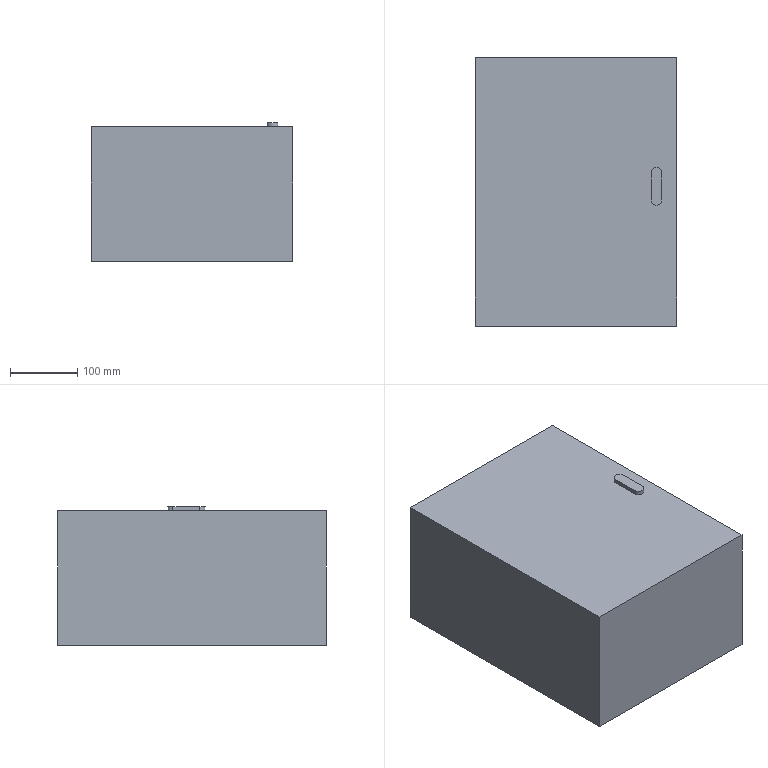Part | SolidWorks | features Extrusion 1, ICE 1 | 1 solid | 11 faces | box 300 x 400 x 206 mm | volume 24005084 mm3 | plane 9 | cylinder 2 | commonest cylinder face diameters 16.06 x2
STEP:
#1=CARTESIAN_POINT('',(-150.,200.,100.));
#2=VERTEX_POINT('',#1);
#3=CARTESIAN_POINT('',(-150.,-200.,100.));
#4=VERTEX_POINT('',#3);
#5=CARTESIAN_POINT('',(-150.,-200.,100.));
#6=DIRECTION('',(0.,-1.,0.));
#7=VECTOR('',#6,1000.);
#8=LINE('',#5,#7);
#9=EDGE_CURVE('',#2,#4,#8,.T.);
#10=ORIENTED_EDGE('',*,*,#9,.T.);
#11=CARTESIAN_POINT('',(150.,-200.,100.));
#12=VERTEX_POINT('',#11);
#13=CARTESIAN_POINT('',(150.,-200.,100.));
#14=DIRECTION('',(1.,0.,0.));
#15=VECTOR('',#14,1000.);
#16=LINE('',#13,#15);
#17=EDGE_CURVE('',#4,#12,#16,.T.);
#18=ORIENTED_EDGE('',*,*,#17,.T.);
#19=CARTESIAN_POINT('',(150.,200.,100.));
#20=VERTEX_POINT('',#19);
#21=CARTESIAN_POINT('',(150.,-200.,100.));
#22=DIRECTION('',(0.,1.,0.));
#23=VECTOR('',#22,1000.);
#24=LINE('',#21,#23);
#25=EDGE_CURVE('',#12,#20,#24,.T.);
#26=ORIENTED_EDGE('',*,*,#25,.T.);
#27=CARTESIAN_POINT('',(150.,200.,100.));
#28=DIRECTION('',(-1.,0.,0.));
#29=VECTOR('',#28,1000.);
#30=LINE('',#27,#29);
#31=EDGE_CURVE('',#20,#2,#30,.T.);
#32=ORIENTED_EDGE('',*,*,#31,.T.);
#33=EDGE_LOOP('',(#10,#18,#26,#32));
#34=FACE_OUTER_BOUND('',#33,.T.);
#35=CARTESIAN_POINT('',(111.97,28.454,100.));
#36=VERTEX_POINT('',#35);
#37=CARTESIAN_POINT('',(111.97,-11.696,100.));
#38=VERTEX_POINT('',#37);
#39=CARTESIAN_POINT('',(111.97,28.454,100.));
#40=DIRECTION('',(0.,-1.,0.));
#41=VECTOR('',#40,1000.);
#42=LINE('',#39,#41);
#43=EDGE_CURVE('',#36,#38,#42,.T.);
#44=ORIENTED_EDGE('',*,*,#43,.F.);
#45=CARTESIAN_POINT('',(128.03,28.454,100.));
#46=VERTEX_POINT('',#45);
#47=CARTESIAN_POINT('',(120.,28.454,100.));
#48=DIRECTION('',(0.,0.,1.));
#49=DIRECTION('',(1.,0.,0.));
#50=AXIS2_PLACEMENT_3D('',#47,#48,#49);
#51=CIRCLE('',#50,8.03);
#52=EDGE_CURVE('',#46,#36,#51,.T.);
#53=ORIENTED_EDGE('',*,*,#52,.F.);
#54=CARTESIAN_POINT('',(128.03,-11.696,100.));
#55=VERTEX_POINT('',#54);
#56=CARTESIAN_POINT('',(128.03,28.454,100.));
#57=DIRECTION('',(0.,1.,0.));
#58=VECTOR('',#57,1000.);
#59=LINE('',#56,#58);
#60=EDGE_CURVE('',#55,#46,#59,.T.);
#61=ORIENTED_EDGE('',*,*,#60,.F.);
#62=CARTESIAN_POINT('',(120.,-11.696,100.));
#63=DIRECTION('',(0.,0.,1.));
#64=DIRECTION('',(1.,0.,0.));
#65=AXIS2_PLACEMENT_3D('',#62,#63,#64);
#66=CIRCLE('',#65,8.03);
#67=EDGE_CURVE('',#38,#55,#66,.T.);
#68=ORIENTED_EDGE('',*,*,#67,.F.);
#69=EDGE_LOOP('',(#44,#53,#61,#68));
#70=FACE_BOUND('',#69,.T.);
#71=CARTESIAN_POINT('',(0.,0.,100.));
#72=DIRECTION('',(0.,0.,1.));
#73=DIRECTION('',(1.,0.,0.));
#74=AXIS2_PLACEMENT_3D('',#71,#72,#73);
#75=PLANE('',#74);
#76=ADVANCED_FACE('',(#34,#70),#75,.T.);
#77=CARTESIAN_POINT('',(-150.,200.,-100.));
#78=VERTEX_POINT('',#77);
#79=CARTESIAN_POINT('',(-150.,-200.,-100.));
#80=VERTEX_POINT('',#79);
#81=CARTESIAN_POINT('',(-150.,-200.,-100.));
#82=DIRECTION('',(0.,-1.,0.));
#83=VECTOR('',#82,1000.);
#84=LINE('',#81,#83);
#85=EDGE_CURVE('',#78,#80,#84,.T.);
#86=ORIENTED_EDGE('',*,*,#85,.T.);
#87=CARTESIAN_POINT('',(-150.,-200.,100.));
#88=DIRECTION('',(0.,0.,-1.));
#89=VECTOR('',#88,1000.);
#90=LINE('',#87,#89);
#91=EDGE_CURVE('',#4,#80,#90,.T.);
#92=ORIENTED_EDGE('',*,*,#91,.F.);
#93=ORIENTED_EDGE('',*,*,#9,.F.);
#94=CARTESIAN_POINT('',(-150.,200.,100.));
#95=DIRECTION('',(0.,0.,-1.));
#96=VECTOR('',#95,1000.);
#97=LINE('',#94,#96);
#98=EDGE_CURVE('',#2,#78,#97,.T.);
#99=ORIENTED_EDGE('',*,*,#98,.T.);
#100=EDGE_LOOP('',(#86,#92,#93,#99));
#101=FACE_OUTER_BOUND('',#100,.T.);
#102=CARTESIAN_POINT('',(-150.,-200.,100.));
#103=DIRECTION('',(1.,0.,0.));
#104=DIRECTION('',(0.,0.,-1.));
#105=AXIS2_PLACEMENT_3D('',#102,#103,#104);
#106=PLANE('',#105);
#107=ADVANCED_FACE('',(#101),#106,.F.);
#108=CARTESIAN_POINT('',(150.,-200.,-100.));
#109=VERTEX_POINT('',#108);
#110=CARTESIAN_POINT('',(150.,-200.,-100.));
#111=DIRECTION('',(1.,0.,0.));
#112=VECTOR('',#111,1000.);
#113=LINE('',#110,#112);
#114=EDGE_CURVE('',#80,#109,#113,.T.);
#115=ORIENTED_EDGE('',*,*,#114,.T.);
#116=CARTESIAN_POINT('',(150.,-200.,100.));
#117=DIRECTION('',(0.,0.,-1.));
#118=VECTOR('',#117,1000.);
#119=LINE('',#116,#118);
#120=EDGE_CURVE('',#12,#109,#119,.T.);
#121=ORIENTED_EDGE('',*,*,#120,.F.);
#122=ORIENTED_EDGE('',*,*,#17,.F.);
#123=ORIENTED_EDGE('',*,*,#91,.T.);
#124=EDGE_LOOP('',(#115,#121,#122,#123));
#125=FACE_OUTER_BOUND('',#124,.T.);
#126=CARTESIAN_POINT('',(150.,-200.,100.));
#127=DIRECTION('',(0.,1.,0.));
#128=DIRECTION('',(-1.,0.,0.));
#129=AXIS2_PLACEMENT_3D('',#126,#127,#128);
#130=PLANE('',#129);
#131=ADVANCED_FACE('',(#125),#130,.F.);
#132=CARTESIAN_POINT('',(150.,200.,-100.));
#133=VERTEX_POINT('',#132);
#134=CARTESIAN_POINT('',(150.,-200.,-100.));
#135=DIRECTION('',(0.,1.,0.));
#136=VECTOR('',#135,1000.);
#137=LINE('',#134,#136);
#138=EDGE_CURVE('',#109,#133,#137,.T.);
#139=ORIENTED_EDGE('',*,*,#138,.T.);
#140=CARTESIAN_POINT('',(150.,200.,100.));
#141=DIRECTION('',(0.,0.,-1.));
#142=VECTOR('',#141,1000.);
#143=LINE('',#140,#142);
#144=EDGE_CURVE('',#20,#133,#143,.T.);
#145=ORIENTED_EDGE('',*,*,#144,.F.);
#146=ORIENTED_EDGE('',*,*,#25,.F.);
#147=ORIENTED_EDGE('',*,*,#120,.T.);
#148=EDGE_LOOP('',(#139,#145,#146,#147));
#149=FACE_OUTER_BOUND('',#148,.T.);
#150=CARTESIAN_POINT('',(150.,-200.,100.));
#151=DIRECTION('',(-1.,0.,0.));
#152=DIRECTION('',(0.,0.,1.));
#153=AXIS2_PLACEMENT_3D('',#150,#151,#152);
#154=PLANE('',#153);
#155=ADVANCED_FACE('',(#149),#154,.F.);
#156=CARTESIAN_POINT('',(150.,200.,-100.));
#157=DIRECTION('',(-1.,0.,0.));
#158=VECTOR('',#157,1000.);
#159=LINE('',#156,#158);
#160=EDGE_CURVE('',#133,#78,#159,.T.);
#161=ORIENTED_EDGE('',*,*,#160,.T.);
#162=ORIENTED_EDGE('',*,*,#98,.F.);
#163=ORIENTED_EDGE('',*,*,#31,.F.);
#164=ORIENTED_EDGE('',*,*,#144,.T.);
#165=EDGE_LOOP('',(#161,#162,#163,#164));
#166=FACE_OUTER_BOUND('',#165,.T.);
#167=CARTESIAN_POINT('',(150.,200.,100.));
#168=DIRECTION('',(0.,-1.,0.));
#169=DIRECTION('',(1.,0.,0.));
#170=AXIS2_PLACEMENT_3D('',#167,#168,#169);
#171=PLANE('',#170);
#172=ADVANCED_FACE('',(#166),#171,.F.);
#173=ORIENTED_EDGE('',*,*,#85,.F.);
#174=ORIENTED_EDGE('',*,*,#160,.F.);
#175=ORIENTED_EDGE('',*,*,#138,.F.);
#176=ORIENTED_EDGE('',*,*,#114,.F.);
#177=EDGE_LOOP('',(#173,#174,#175,#176));
#178=FACE_OUTER_BOUND('',#177,.T.);
#179=CARTESIAN_POINT('',(0.,0.,-100.));
#180=DIRECTION('',(0.,0.,1.));
#181=DIRECTION('',(1.,0.,0.));
#182=AXIS2_PLACEMENT_3D('',#179,#180,#181);
#183=PLANE('',#182);
#184=ADVANCED_FACE('',(#178),#183,.F.);
#185=ORIENTED_EDGE('',*,*,#52,.T.);
#186=CARTESIAN_POINT('',(111.97,28.454,106.));
#187=VERTEX_POINT('',#186);
#188=CARTESIAN_POINT('',(111.97,28.454,106.));
#189=DIRECTION('',(0.,0.,-1.));
#190=VECTOR('',#189,1000.);
#191=LINE('',#188,#190);
#192=EDGE_CURVE('',#187,#36,#191,.T.);
#193=ORIENTED_EDGE('',*,*,#192,.F.);
#194=CARTESIAN_POINT('',(128.03,28.454,106.));
#195=VERTEX_POINT('',#194);
#196=CARTESIAN_POINT('',(120.,28.454,106.));
#197=DIRECTION('',(0.,0.,1.));
#198=DIRECTION('',(1.,0.,0.));
#199=AXIS2_PLACEMENT_3D('',#196,#197,#198);
#200=CIRCLE('',#199,8.03);
#201=EDGE_CURVE('',#195,#187,#200,.T.);
#202=ORIENTED_EDGE('',*,*,#201,.F.);
#203=CARTESIAN_POINT('',(128.03,28.454,106.));
#204=DIRECTION('',(0.,0.,-1.));
#205=VECTOR('',#204,1000.);
#206=LINE('',#203,#205);
#207=EDGE_CURVE('',#195,#46,#206,.T.);
#208=ORIENTED_EDGE('',*,*,#207,.T.);
#209=EDGE_LOOP('',(#185,#193,#202,#208));
#210=FACE_OUTER_BOUND('',#209,.T.);
#211=CARTESIAN_POINT('',(120.,28.454,106.));
#212=DIRECTION('',(0.,0.,-1.));
#213=DIRECTION('',(-1.,0.,0.));
#214=AXIS2_PLACEMENT_3D('',#211,#212,#213);
#215=CYLINDRICAL_SURFACE('',#214,8.03);
#216=ADVANCED_FACE('',(#210),#215,.T.);
#217=ORIENTED_EDGE('',*,*,#43,.T.);
#218=CARTESIAN_POINT('',(111.97,-11.696,106.));
#219=VERTEX_POINT('',#218);
#220=CARTESIAN_POINT('',(111.97,-11.696,106.));
#221=DIRECTION('',(0.,0.,-1.));
#222=VECTOR('',#221,1000.);
#223=LINE('',#220,#222);
#224=EDGE_CURVE('',#219,#38,#223,.T.);
#225=ORIENTED_EDGE('',*,*,#224,.F.);
#226=CARTESIAN_POINT('',(111.97,28.454,106.));
#227=DIRECTION('',(0.,-1.,0.));
#228=VECTOR('',#227,1000.);
#229=LINE('',#226,#228);
#230=EDGE_CURVE('',#187,#219,#229,.T.);
#231=ORIENTED_EDGE('',*,*,#230,.F.);
#232=ORIENTED_EDGE('',*,*,#192,.T.);
#233=EDGE_LOOP('',(#217,#225,#231,#232));
#234=FACE_OUTER_BOUND('',#233,.T.);
#235=CARTESIAN_POINT('',(111.97,28.454,106.));
#236=DIRECTION('',(1.,0.,0.));
#237=DIRECTION('',(0.,1.,0.));
#238=AXIS2_PLACEMENT_3D('',#235,#236,#237);
#239=PLANE('',#238);
#240=ADVANCED_FACE('',(#234),#239,.F.);
#241=ORIENTED_EDGE('',*,*,#67,.T.);
#242=CARTESIAN_POINT('',(128.03,-11.696,106.));
#243=VERTEX_POINT('',#242);
#244=CARTESIAN_POINT('',(128.03,-11.696,106.));
#245=DIRECTION('',(0.,0.,-1.));
#246=VECTOR('',#245,1000.);
#247=LINE('',#244,#246);
#248=EDGE_CURVE('',#243,#55,#247,.T.);
#249=ORIENTED_EDGE('',*,*,#248,.F.);
#250=CARTESIAN_POINT('',(120.,-11.696,106.));
#251=DIRECTION('',(0.,0.,1.));
#252=DIRECTION('',(1.,0.,0.));
#253=AXIS2_PLACEMENT_3D('',#250,#251,#252);
#254=CIRCLE('',#253,8.03);
#255=EDGE_CURVE('',#219,#243,#254,.T.);
#256=ORIENTED_EDGE('',*,*,#255,.F.);
#257=ORIENTED_EDGE('',*,*,#224,.T.);
#258=EDGE_LOOP('',(#241,#249,#256,#257));
#259=FACE_OUTER_BOUND('',#258,.T.);
#260=CARTESIAN_POINT('',(120.,-11.696,106.));
#261=DIRECTION('',(0.,0.,-1.));
#262=DIRECTION('',(-1.,0.,0.));
#263=AXIS2_PLACEMENT_3D('',#260,#261,#262);
#264=CYLINDRICAL_SURFACE('',#263,8.03);
#265=ADVANCED_FACE('',(#259),#264,.T.);
#266=ORIENTED_EDGE('',*,*,#60,.T.);
#267=ORIENTED_EDGE('',*,*,#207,.F.);
#268=CARTESIAN_POINT('',(128.03,28.454,106.));
#269=DIRECTION('',(0.,1.,0.));
#270=VECTOR('',#269,1000.);
#271=LINE('',#268,#270);
#272=EDGE_CURVE('',#243,#195,#271,.T.);
#273=ORIENTED_EDGE('',*,*,#272,.F.);
#274=ORIENTED_EDGE('',*,*,#248,.T.);
#275=EDGE_LOOP('',(#266,#267,#273,#274));
#276=FACE_OUTER_BOUND('',#275,.T.);
#277=CARTESIAN_POINT('',(128.03,28.454,106.));
#278=DIRECTION('',(-1.,0.,0.));
#279=DIRECTION('',(0.,-1.,0.));
#280=AXIS2_PLACEMENT_3D('',#277,#278,#279);
#281=PLANE('',#280);
#282=ADVANCED_FACE('',(#276),#281,.F.);
#283=ORIENTED_EDGE('',*,*,#201,.T.);
#284=ORIENTED_EDGE('',*,*,#230,.T.);
#285=ORIENTED_EDGE('',*,*,#255,.T.);
#286=ORIENTED_EDGE('',*,*,#272,.T.);
#287=EDGE_LOOP('',(#283,#284,#285,#286));
#288=FACE_OUTER_BOUND('',#287,.T.);
#289=CARTESIAN_POINT('',(120.,28.454,106.));
#290=DIRECTION('',(0.,0.,1.));
#291=DIRECTION('',(1.,0.,0.));
#292=AXIS2_PLACEMENT_3D('',#289,#290,#291);
#293=PLANE('',#292);
#294=ADVANCED_FACE('',(#288),#293,.T.);
#295=CLOSED_SHELL('',(#76,#107,#131,#155,#172,#184,#216,#240,#265,#282,#294));
#296=MANIFOLD_SOLID_BREP('',#295);
#297=CARTESIAN_POINT('',(0.,0.,0.));
#298=DIRECTION('',(0.,0.,1.));
#299=DIRECTION('',(1.,0.,0.));
#300=AXIS2_PLACEMENT_3D('',#297,#298,#299);
#301=(LENGTH_UNIT()NAMED_UNIT(*)SI_UNIT(.MILLI.,.METRE.));
#302=UNCERTAINTY_MEASURE_WITH_UNIT(LENGTH_MEASURE(0.00001),#301,'','');
#303=(NAMED_UNIT(*)PLANE_ANGLE_UNIT()SI_UNIT($,.RADIAN.));
#304=(NAMED_UNIT(*)SI_UNIT($,.STERADIAN.)SOLID_ANGLE_UNIT());
#305=(GEOMETRIC_REPRESENTATION_CONTEXT(3)GLOBAL_UNCERTAINTY_ASSIGNED_CONTEXT((#302))GLOBAL_UNIT_ASSIGNED_CONTEXT((#301,#303,#304))REPRESENTATION_CONTEXT('',''));
#306=ADVANCED_BREP_SHAPE_REPRESENTATION('',(#296,#300),#305);